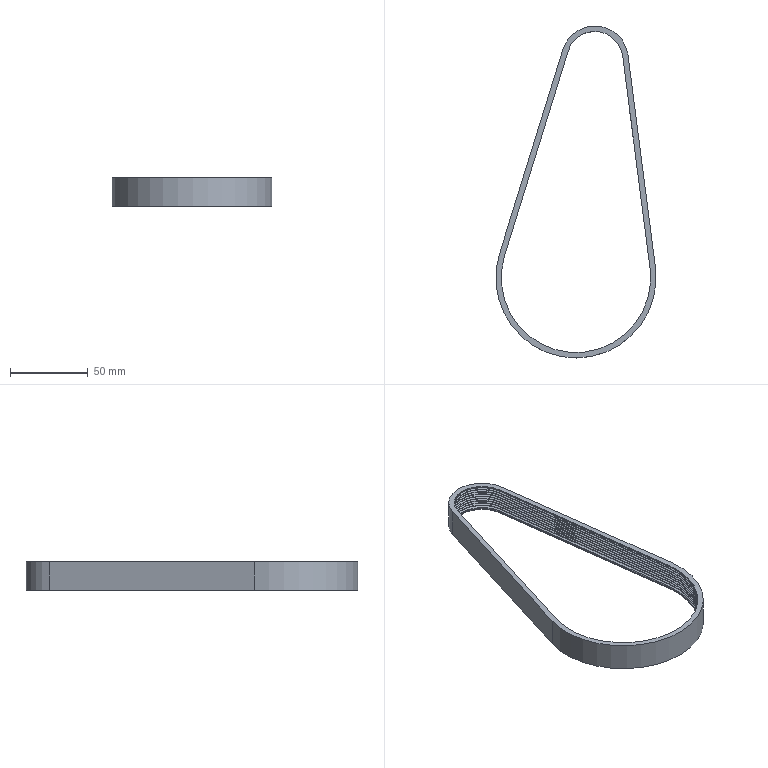Part | STEP file | DE200JNQ7A | 1 solid | 234 faces | box 103 x 213.3 x 18 mm | volume 21815 mm3 | cylinder 80 | plane 62 | torus 56 | cone 36 | commonest cylinder face diameters 0.4 x52 40 x9 100 x9 1 x4 36 x2 96 x2